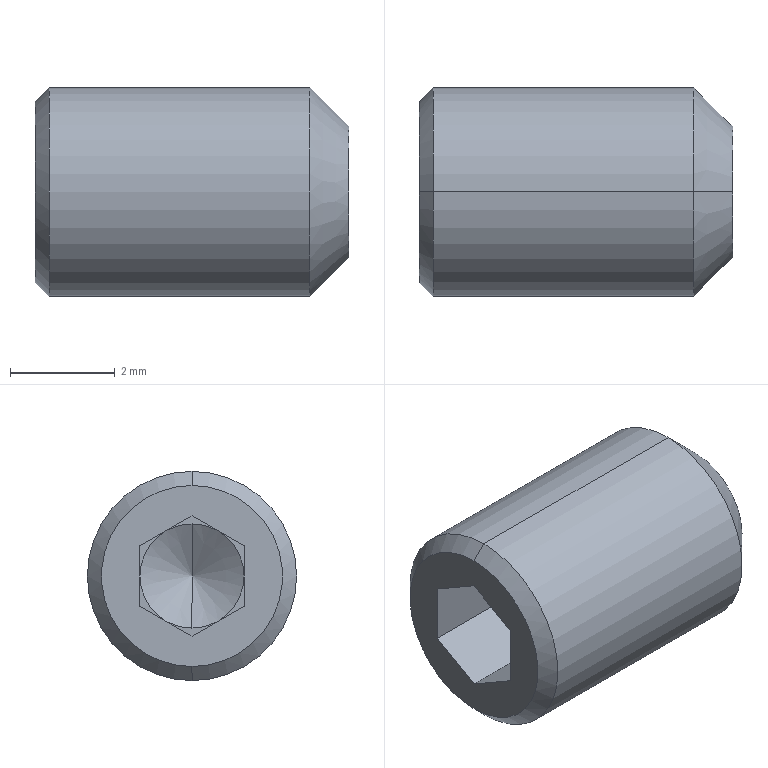Part | SolidWorks | features RevCut 2, Cut 1, LPattern 1, Revolution 1 | 1 solid | 22 faces | box 6 x 4 x 4 mm | volume 66.123 mm3 | plane 14 | cone 6 | cylinder 2 | commonest cylinder face diameters 4 x2